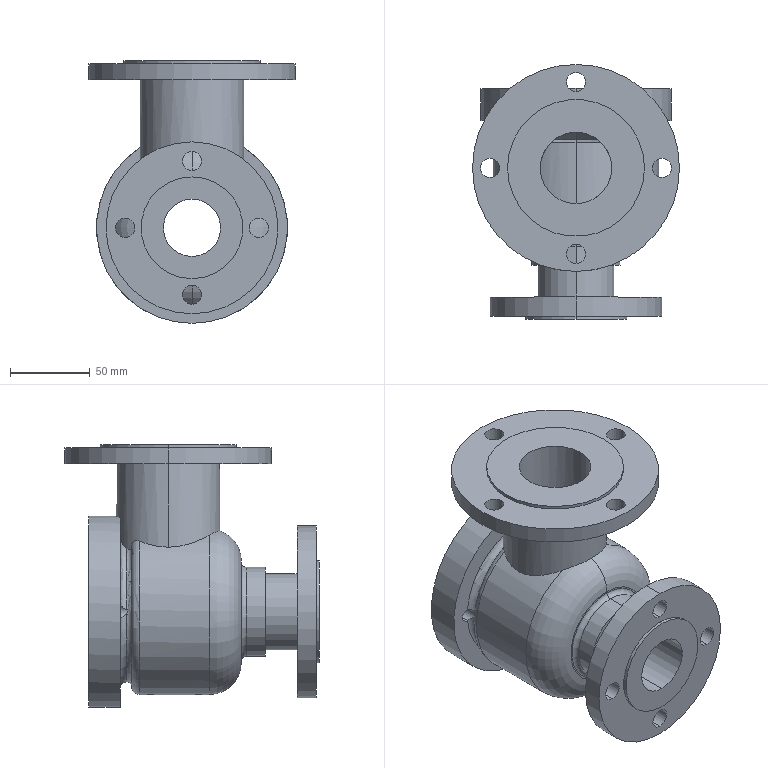Part | SolidWorks | features ICE 3, HoleWzd 2, Revolution 2, RevCut 1 | 1 solid | 97 faces | box 130 x 160 x 165 mm | volume 638021 mm3 | cylinder 61 | plane 16 | torus 12 | cone 8 | commonest cylinder face diameters 12 x16 8.5 x8 5 x4 104 x3 36 x2 44 x2